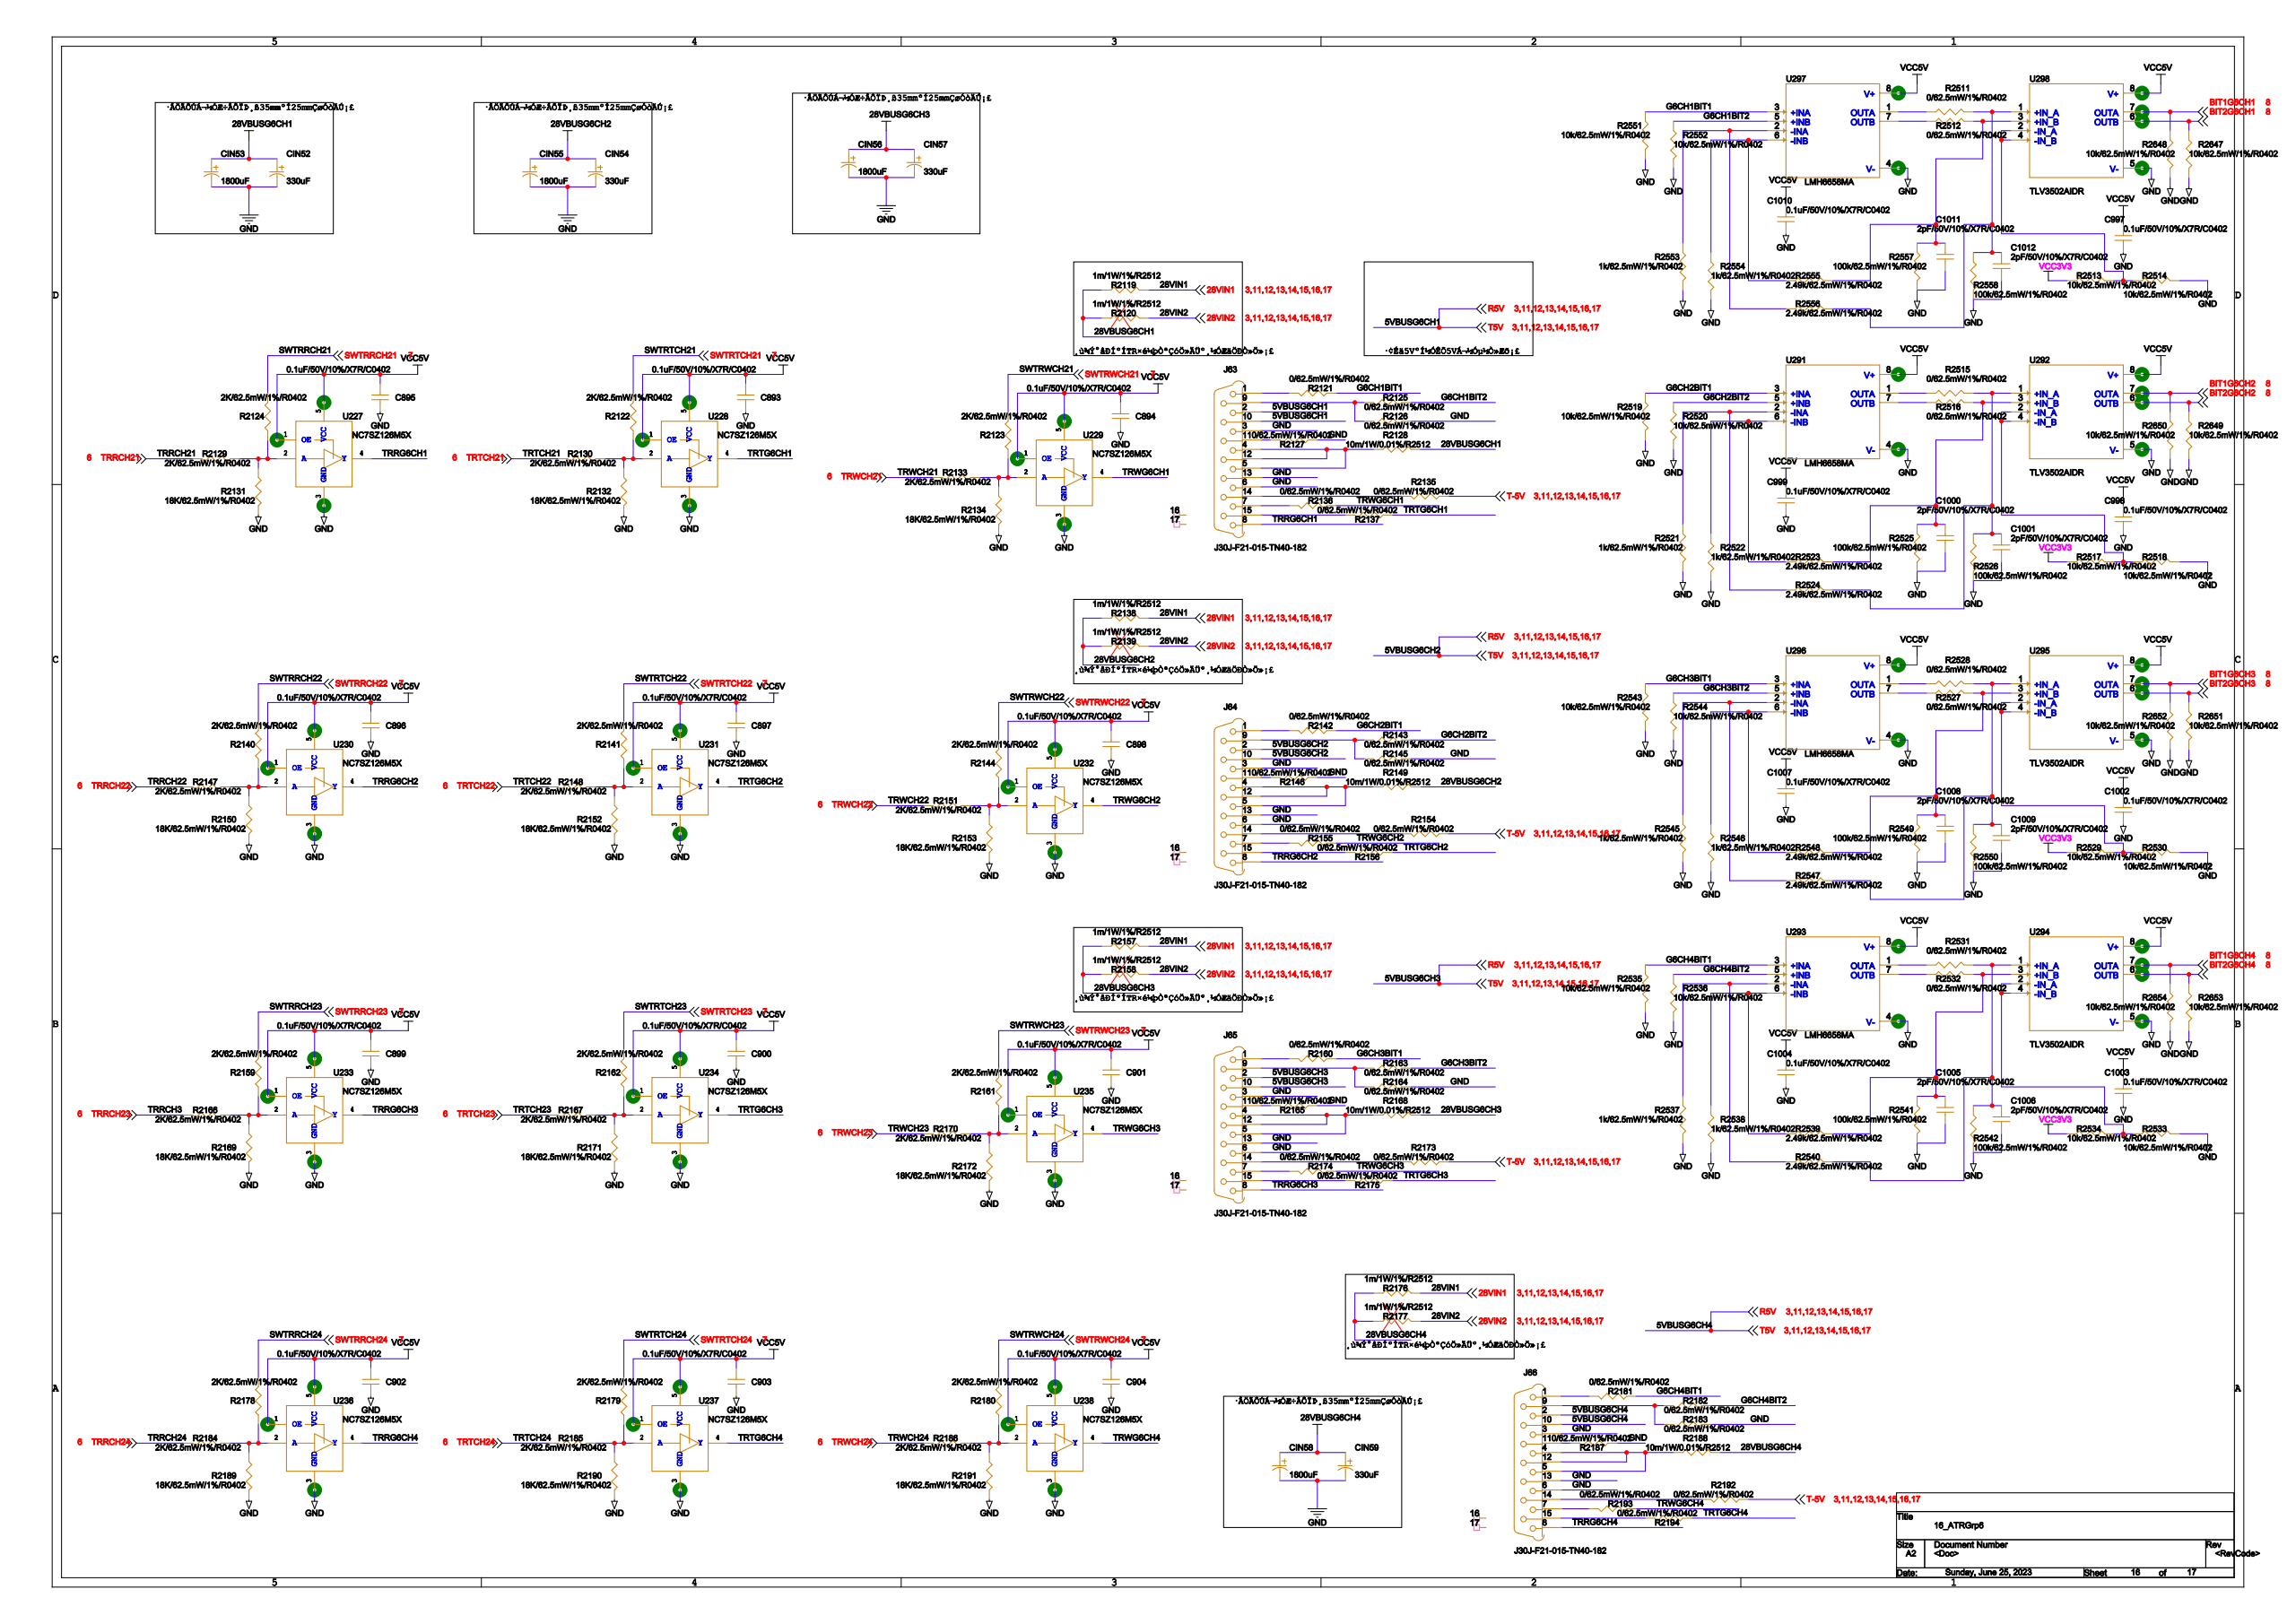Circuit board | Cadence Allegro | 2002 parts | 1538 nets | one sheet of the schematic
Parts on this sheet (reference | value | footprint):
C893 | 0.1uF/50V/10%/X7R/C0402 | 0402
C894 | 0.1uF/50V/10%/X7R/C0402 | 0402
C895 | 0.1uF/50V/10%/X7R/C0402 | 0402
C896 | 0.1uF/50V/10%/X7R/C0402 | 0402
C897 | 0.1uF/50V/10%/X7R/C0402 | 0402
C898 | 0.1uF/50V/10%/X7R/C0402 | 0402
C899 | 0.1uF/50V/10%/X7R/C0402 | 0402
C900 | 0.1uF/50V/10%/X7R/C0402 | 0402
C901 | 0.1uF/50V/10%/X7R/C0402 | 0402
C902 | 0.1uF/50V/10%/X7R/C0402 | 0402
C903 | 0.1uF/50V/10%/X7R/C0402 | 0402
C904 | 0.1uF/50V/10%/X7R/C0402 | 0402
C997 | 0.1uF/50V/10%/X7R/C0402 | 0402
C998 | 0.1uF/50V/10%/X7R/C0402 | 0402
C1000 | 2pF/50V/10%/X7R/C0402 | 0402
C1001 | 2pF/50V/10%/X7R/C0402 | 0402
C1002 | 0.1uF/50V/10%/X7R/C0402 | 0402
C1003 | 0.1uF/50V/10%/X7R/C0402 | 0402
C1005 | 2pF/50V/10%/X7R/C0402 | 0402
C1006 | 2pF/50V/10%/X7R/C0402 | 0402
C1008 | 2pF/50V/10%/X7R/C0402 | 0402
C1009 | 2pF/50V/10%/X7R/C0402 | 0402
C1011 | 2pF/50V/10%/X7R/C0402 | 0402
C1012 | 2pF/50V/10%/X7R/C0402 | 0402
CIN52 | ECF1JM331G20OTPO | AP-SMD_BD10-L20-W6_6-LS7_21
CIN53 | ECF1HM182M27OTPO | AP-SMD_BD18-L27-W6_6-LS7_21
CIN54 | ECF1JM331G20OTPO | AP-SMD_BD10-L20-W6_6-LS7_21
CIN55 | ECF1HM182M27OTPO | AP-SMD_BD18-L27-W6_6-LS7_21
CIN56 | ECF1HM182M27OTPO | AP-SMD_BD18-L27-W6_6-LS7_21
CIN57 | ECF1JM331G20OTPO | AP-SMD_BD10-L20-W6_6-LS7_21
CIN58 | ECF1HM182M27OTPO | AP-SMD_BD18-L27-W6_6-LS7_21
CIN59 | ECF1JM331G20OTPO | AP-SMD_BD10-L20-W6_6-LS7_21
J63 | J30J-F21-015-TN40-182 | J30J-F21-015-TN40-182
J64 | J30J-F21-015-TN40-182 | J30J-F21-015-TN40-182
J65 | J30J-F21-015-TN40-182 | J30J-F21-015-TN40-182
J66 | J30J-F21-015-TN40-182 | J30J-F21-015-TN40-182
R2119 | 1m/1W/1%/R2512 | 2512
R2120 | 1m/1W/1%/R2512 | 2512
R2121 | 0/62.5mW/1%/R0402 | 0402
R2122 | 2K/62.5mW/1%/R0402 | 0402
R2123 | 2K/62.5mW/1%/R0402 | 0402
R2124 | 2K/62.5mW/1%/R0402 | 0402
R2125 | 0/62.5mW/1%/R0402 | 0402
R2126 | 0/62.5mW/1%/R0402 | 0402
R2127 | 0/62.5mW/1%/R0402 | 0402
R2128 | 10m/1W/0.01%/R2512 | 2512
R2129 | 2K/62.5mW/1%/R0402 | 0402
R2130 | 2K/62.5mW/1%/R0402 | 0402
R2131 | 18K/62.5mW/1%/R0402 | 0402
R2132 | 18K/62.5mW/1%/R0402 | 0402
R2133 | 2K/62.5mW/1%/R0402 | 0402
R2134 | 18K/62.5mW/1%/R0402 | 0402
R2135 | 0/62.5mW/1%/R0402 | 0402
R2136 | 0/62.5mW/1%/R0402 | 0402
R2137 | 0/62.5mW/1%/R0402 | 0402
R2138 | 1m/1W/1%/R2512 | 2512
R2139 | 1m/1W/1%/R2512 | 2512
R2140 | 2K/62.5mW/1%/R0402 | 0402
R2141 | 2K/62.5mW/1%/R0402 | 0402
R2142 | 0/62.5mW/1%/R0402 | 0402
R2143 | 0/62.5mW/1%/R0402 | 0402
R2144 | 2K/62.5mW/1%/R0402 | 0402
R2145 | 0/62.5mW/1%/R0402 | 0402
R2146 | 0/62.5mW/1%/R0402 | 0402
R2147 | 2K/62.5mW/1%/R0402 | 0402
R2148 | 2K/62.5mW/1%/R0402 | 0402
R2149 | 10m/1W/0.01%/R2512 | 2512
R2150 | 18K/62.5mW/1%/R0402 | 0402
R2151 | 2K/62.5mW/1%/R0402 | 0402
R2152 | 18K/62.5mW/1%/R0402 | 0402
R2153 | 18K/62.5mW/1%/R0402 | 0402
R2154 | 0/62.5mW/1%/R0402 | 0402
R2155 | 0/62.5mW/1%/R0402 | 0402
R2156 | 0/62.5mW/1%/R0402 | 0402
R2157 | 1m/1W/1%/R2512 | 2512
R2158 | 1m/1W/1%/R2512 | 2512
R2159 | 2K/62.5mW/1%/R0402 | 0402
R2160 | 0/62.5mW/1%/R0402 | 0402
R2161 | 2K/62.5mW/1%/R0402 | 0402
R2162 | 2K/62.5mW/1%/R0402 | 0402
R2163 | 0/62.5mW/1%/R0402 | 0402
R2164 | 0/62.5mW/1%/R0402 | 0402
R2165 | 0/62.5mW/1%/R0402 | 0402
R2166 | 2K/62.5mW/1%/R0402 | 0402
R2167 | 2K/62.5mW/1%/R0402 | 0402
R2168 | 10m/1W/0.01%/R2512 | 2512
R2169 | 18K/62.5mW/1%/R0402 | 0402
R2170 | 2K/62.5mW/1%/R0402 | 0402
R2171 | 18K/62.5mW/1%/R0402 | 0402
R2172 | 18K/62.5mW/1%/R0402 | 0402
R2173 | 0/62.5mW/1%/R0402 | 0402
R2174 | 0/62.5mW/1%/R0402 | 0402
R2175 | 0/62.5mW/1%/R0402 | 0402
R2176 | 1m/1W/1%/R2512 | 2512
R2177 | 1m/1W/1%/R2512 | 2512
R2178 | 2K/62.5mW/1%/R0402 | 0402
R2179 | 2K/62.5mW/1%/R0402 | 0402
R2180 | 2K/62.5mW/1%/R0402 | 0402
R2181 | 0/62.5mW/1%/R0402 | 0402
R2182 | 0/62.5mW/1%/R0402 | 0402
R2183 | 0/62.5mW/1%/R0402 | 0402
R2184 | 2K/62.5mW/1%/R0402 | 0402
R2185 | 2K/62.5mW/1%/R0402 | 0402
R2186 | 2K/62.5mW/1%/R0402 | 0402
R2187 | 0/62.5mW/1%/R0402 | 0402
R2188 | 10m/1W/0.01%/R2512 | 2512
R2189 | 18K/62.5mW/1%/R0402 | 0402
R2190 | 18K/62.5mW/1%/R0402 | 0402
R2191 | 18K/62.5mW/1%/R0402 | 0402
R2192 | 0/62.5mW/1%/R0402 | 0402
R2193 | 0/62.5mW/1%/R0402 | 0402
R2194 | 0/62.5mW/1%/R0402 | 0402
R2511 | 0/62.5mW/1%/R0402 | 0402
R2512 | 0/62.5mW/1%/R0402 | 0402
R2513 | 10k/62.5mW/1%/R0402 | 0402
R2514 | 10k/62.5mW/1%/R0402 | 0402
R2515 | 0/62.5mW/1%/R0402 | 0402
R2516 | 0/62.5mW/1%/R0402 | 0402
R2517 | 10k/62.5mW/1%/R0402 | 0402
R2518 | 10k/62.5mW/1%/R0402 | 0402
R2519 | 10k/62.5mW/1%/R0402 | 0402
R2520 | 10k/62.5mW/1%/R0402 | 0402
R2521 | 1K/62.5mW/1%/R0402 | 0402
R2522 | 1K/62.5mW/1%/R0402 | 0402
R2524 | 2.49k/62.5mW/1%/R0402 | 0402
R2525 | 100k/62.5mW/1%/R0402 | 0402
R2526 | 100k/62.5mW/1%/R0402 | 0402
R2527 | 0/62.5mW/1%/R0402 | 0402
R2528 | 0/62.5mW/1%/R0402 | 0402
R2529 | 10k/62.5mW/1%/R0402 | 0402
R2530 | 10k/62.5mW/1%/R0402 | 0402
R2531 | 0/62.5mW/1%/R0402 | 0402
R2532 | 0/62.5mW/1%/R0402 | 0402
R2533 | 10k/62.5mW/1%/R0402 | 0402
R2534 | 10k/62.5mW/1%/R0402 | 0402
R2535 | 10k/62.5mW/1%/R0402 | 0402
R2536 | 10k/62.5mW/1%/R0402 | 0402
R2537 | 1K/62.5mW/1%/R0402 | 0402
R2538 | 1K/62.5mW/1%/R0402 | 0402
R2540 | 2.49k/62.5mW/1%/R0402 | 0402
R2541 | 100k/62.5mW/1%/R0402 | 0402
R2542 | 100k/62.5mW/1%/R0402 | 0402
R2543 | 10k/62.5mW/1%/R0402 | 0402
R2544 | 10k/62.5mW/1%/R0402 | 0402
R2545 | 1K/62.5mW/1%/R0402 | 0402
R2546 | 1K/62.5mW/1%/R0402 | 0402
R2547 | 2.49k/62.5mW/1%/R0402 | 0402
R2548 | 2.49k/62.5mW/1%/R0402 | 0402
R2549 | 100k/62.5mW/1%/R0402 | 0402
R2550 | 100k/62.5mW/1%/R0402 | 0402
R2551 | 10k/62.5mW/1%/R0402 | 0402
R2552 | 10k/62.5mW/1%/R0402 | 0402
R2553 | 1K/62.5mW/1%/R0402 | 0402
R2554 | 1K/62.5mW/1%/R0402 | 0402
R2556 | 2.49k/62.5mW/1%/R0402 | 0402
R2557 | 100k/62.5mW/1%/R0402 | 0402
R2558 | 100k/62.5mW/1%/R0402 | 0402
R2647 | 10k/62.5mW/1%/R0402 | 0402
R2648 | 10k/62.5mW/1%/R0402 | 0402
R2649 | 10k/62.5mW/1%/R0402 | 0402
R2650 | 10k/62.5mW/1%/R0402 | 0402
R2651 | 10k/62.5mW/1%/R0402 | 0402
R2652 | 10k/62.5mW/1%/R0402 | 0402
R2653 | 10k/62.5mW/1%/R0402 | 0402
R2654 | 10k/62.5mW/1%/R0402 | 0402
U227 | NC7SZ126M5X | SOT-23-5
U228 | NC7SZ126M5X | SOT-23-5
U229 | NC7SZ126M5X | SOT-23-5
U230 | NC7SZ126M5X | SOT-23-5
U231 | NC7SZ126M5X | SOT-23-5
U232 | NC7SZ126M5X | SOT-23-5
U233 | NC7SZ126M5X | SOT-23-5
U234 | NC7SZ126M5X | SOT-23-5
U235 | NC7SZ126M5X | SOT-23-5
U236 | NC7SZ126M5X | SOT-23-5
U237 | NC7SZ126M5X | SOT-23-5
U238 | NC7SZ126M5X | SOT-23-5
U291 | LMH6658MA | SOIC127P599X175-8N
U293 | LMH6658MA | SOIC127P599X175-8N
U295 | TLV3502AIDR | SOIC127P599X175-8N
U297 | LMH6658MA | SOIC127P599X175-8N
Nets of these parts (net: part-pin ...):
3.3V: R2513-1 R2517-1 R2529-1 R2534-1
AGND: C893-2 C894-2 C895-2 C896-2 C897-2 C898-2 C899-2 C900-2 C901-2 C902-2 C903-2 C904-2 C997-2 C998-2 C1000-2 C1001-2 C1002-2 C1003-2 C1005-2 C1006-2 C1008-2 C1009-2 C1011-2 C1012-2 CIN52-2 CIN53-2 CIN54-2 CIN55-2 CIN56-2 CIN57-2 CIN58-2 CIN59-2 J63-3 J63-6 J63-13 J64-3 J64-6 J64-13 J65-3 J65-6 J65-13 J66-3 J66-6 J66-13 R2126-1 R2127-1 R2131-1 R2132-1 R2134-1 R2145-1 R2146-1 R2150-1 R2152-1 R2153-1 R2164-1 R2165-1 R2169-1 R2171-1 R2172-1 R2183-1 R2187-1 R2189-1 R2190-1 R2191-1 R2514-2 R2518-2 R2519-2 R2520-2 R2521-2 R2522-2 R2525-2 R2526-2 R2530-2 R2533-2 R2535-2 R2536-2 R2537-2 R2538-2 R2541-2 R2542-2 R2543-2 R2544-2 R2545-2 R2546-2 R2549-2 R2550-2 R2551-2 R2552-2 R2553-2 R2554-2 R2557-2 R2558-2 R2647-2 R2648-2 R2649-2 R2650-2 R2651-2 R2652-2 R2653-2 R2654-2 U227-3 U228-3 U229-3 U230-3 U231-3 U232-3 U233-3 U234-3 U235-3 U236-3 U237-3 U238-3 U291-4 U293-4 U295-5 U297-4
VCC5V: C893-1 C894-1 C895-1 C896-1 C897-1 C898-1 C899-1 C900-1 C901-1 C902-1 C903-1 C904-1 C997-1 C998-1 C1002-1 C1003-1 U227-1 U227-5 U228-1 U228-5 U229-1 U229-5 U230-1 U230-5 U231-1 U231-5 U232-1 U232-5 U233-1 U233-5 U234-1 U234-5 U235-1 U235-5 U236-1 U236-5 U237-1 U237-5 U238-1 U238-5 U291-8 U293-8 U295-8 U297-8
28VIN1: R2119-2 R2120-2 R2138-2 R2139-2 R2157-2 R2158-2 R2176-2 R2177-2
R5V: J63-2 J63-10 J64-2 J64-10 J65-2 J65-10 J66-2 J66-10
T-5V: R2135-1 R2154-1 R2173-1 R2192-1
N24409583: R2522-1 U291-6
N24409593: C1000-1 R2516-2 R2525-1
N24409571: R2521-1 R2524-1 U291-2
N24409591: C1001-1 R2515-2 R2524-2 R2526-1
N24410137: R2538-1 U293-6
N24410147: C1005-1 R2532-2 R2541-1
N24410125: R2537-1 R2540-1 U293-2
N24410145: C1006-1 R2531-2 R2540-2 R2542-1
N24409949: R2545-1 R2547-1
N24409965: C1009-1 R2528-2 R2547-2 R2550-1 U295-1
N24409953: R2546-1 R2548-1
N24409967: C1008-1 R2527-2 R2548-2 R2549-1 U295-3
N24409403: R2554-1 U297-6
N24409413: C1011-1 R2512-2 R2557-1
N24409399: R2553-1 R2556-1 U297-2
N24409411: C1012-1 R2511-2 R2556-2 R2558-1
G6CH2BIT1: R2142-1 R2519-1 U291-3
G6CH2BIT2: R2143-1 R2520-1 U291-5
N24409587: R2515-1 U291-1
N24409589: R2516-1 U291-7
G6CH4BIT1: R2181-1 R2535-1 U293-3
G6CH4BIT2: R2182-1 R2536-1 U293-5
N24410141: R2531-1 U293-1
N24410143: R2532-1 U293-7
G6CH3BIT1: R2160-1 R2543-1
G6CH3BIT2: R2163-1 R2544-1
N24409961: R2528-1
N24409963: R2527-1
G6CH1BIT1: R2121-1 R2551-1 U297-3
G6CH1BIT2: R2125-1 R2552-1 U297-5
N24409407: R2511-1 U297-1
N24409409: R2512-1 U297-7
N24409645: R2517-2 R2518-1
BIT1G6CH2: R2650-1
BIT2G6CH2: R2649-1
N24410199: R2533-1 R2534-2
BIT1G6CH4: R2654-1
BIT2G6CH4: R2653-1
N24410019: R2529-2 R2530-1 U295-2 U295-4
BIT1G6CH3: R2652-1 U295-7
BIT2G6CH3: R2651-1 U295-6
N24409465: R2513-2 R2514-1
BIT1G6CH1: R2648-1
BIT2G6CH1: R2647-1
N23733637: J63-1 R2121-2
N23733650: J63-11 R2127-2
N23733652: J63-4 J63-5 J63-12 R2128-1
N23733664: J63-14 R2135-2
N23733668: J63-15 R2137-2
N23733666: J63-7 R2136-2
TRRG6CH1: J63-8 U227-4
N23733639: J63-9 R2125-2 R2126-2
N23734196: J64-1 R2142-2
N23734209: J64-11 R2146-2
N23734211: J64-4 J64-5 J64-12 R2149-1
N23734223: J64-14 R2154-2
N23734227: J64-15 R2156-2
N23734225: J64-7 R2155-2
TRRG6CH2: J64-8 U230-4
N23734198: J64-9 R2143-2 R2145-2
N23734823: J65-1 R2160-2
N23734836: J65-11 R2165-2
N23734838: J65-4 J65-5 J65-12 R2168-1
N23734850: J65-14 R2173-2
N23734854: J65-15 R2175-2
N23734852: J65-7 R2174-2
TRRG6CH3: J65-8 U233-4
N23734825: J65-9 R2163-2 R2164-2
N23735455: J66-1 R2181-2
N23735468: J66-11 R2187-2
N23735470: J66-4 J66-5 J66-12 R2188-1
N23735482: J66-14 R2192-2
N23735486: J66-15 R2194-2
N23735484: J66-7 R2193-2
TRRG6CH4: J66-8 U236-4
N23735457: J66-9 R2182-2 R2183-2
28VBUSG6CH1: CIN52-1 CIN53-1 R2119-1 R2120-1 R2128-2
28VBUSG6CH2: CIN54-1 CIN55-1 R2138-1 R2139-1 R2149-2
28VBUSG6CH3: CIN56-1 CIN57-1 R2157-1 R2158-1 R2168-2
28VBUSG6CH4: CIN58-1 CIN59-1 R2176-1 R2177-1 R2188-2
SWTRTCH21: R2122-1
N24017305: R2122-2 R2130-2 R2132-2 U228-2
SWTRWCH21: R2123-1
N24017793: R2123-2 R2133-2 R2134-2 U229-2
SWTRRCH21: R2124-1
N24018285: R2124-2 R2129-2 R2131-2 U227-2
TRRCH21: R2129-1
TRTCH21: R2130-1
TRWCH21: R2133-1
SWTRRCH22: R2140-1
N24018403: R2140-2 R2147-2 R2150-2 U230-2
SWTRTCH22: R2141-1
N24017423: R2141-2 R2148-2 R2152-2 U231-2
SWTRWCH22: R2144-1
N24017915: R2144-2 R2151-2 R2153-2 U232-2
TRRCH22: R2147-1
TRTCH22: R2148-1
TRWCH22: R2151-1
SWTRRCH23: R2159-1
N24018529: R2159-2 R2166-2 R2169-2 U233-2
SWTRWCH23: R2161-1
N24018037: R2161-2 R2170-2 R2172-2 U235-2
SWTRTCH23: R2162-1
N24017549: R2162-2 R2167-2 R2171-2 U234-2
TRRCH23: R2166-1
TRTCH23: R2167-1
TRWCH23: R2170-1
SWTRRCH24: R2178-1
N24018647: R2178-2 R2184-2 R2189-2 U236-2
SWTRTCH24: R2179-1
N24017671: R2179-2 R2185-2 R2190-2 U237-2
SWTRWCH24: R2180-1
N24018159: R2180-2 R2186-2 R2191-2 U238-2
TRRCH24: R2184-1
TRTCH24: R2185-1
TRWCH24: R2186-1
TRTG6CH1: R2137-1 U228-4
TRWG6CH1: R2136-1 U229-4
TRTG6CH2: R2156-1 U231-4
TRWG6CH2: R2155-1 U232-4
TRTG6CH3: R2175-1 U234-4
TRWG6CH3: R2174-1 U235-4
TRTG6CH4: R2194-1 U237-4
TRWG6CH4: R2193-1 U238-4